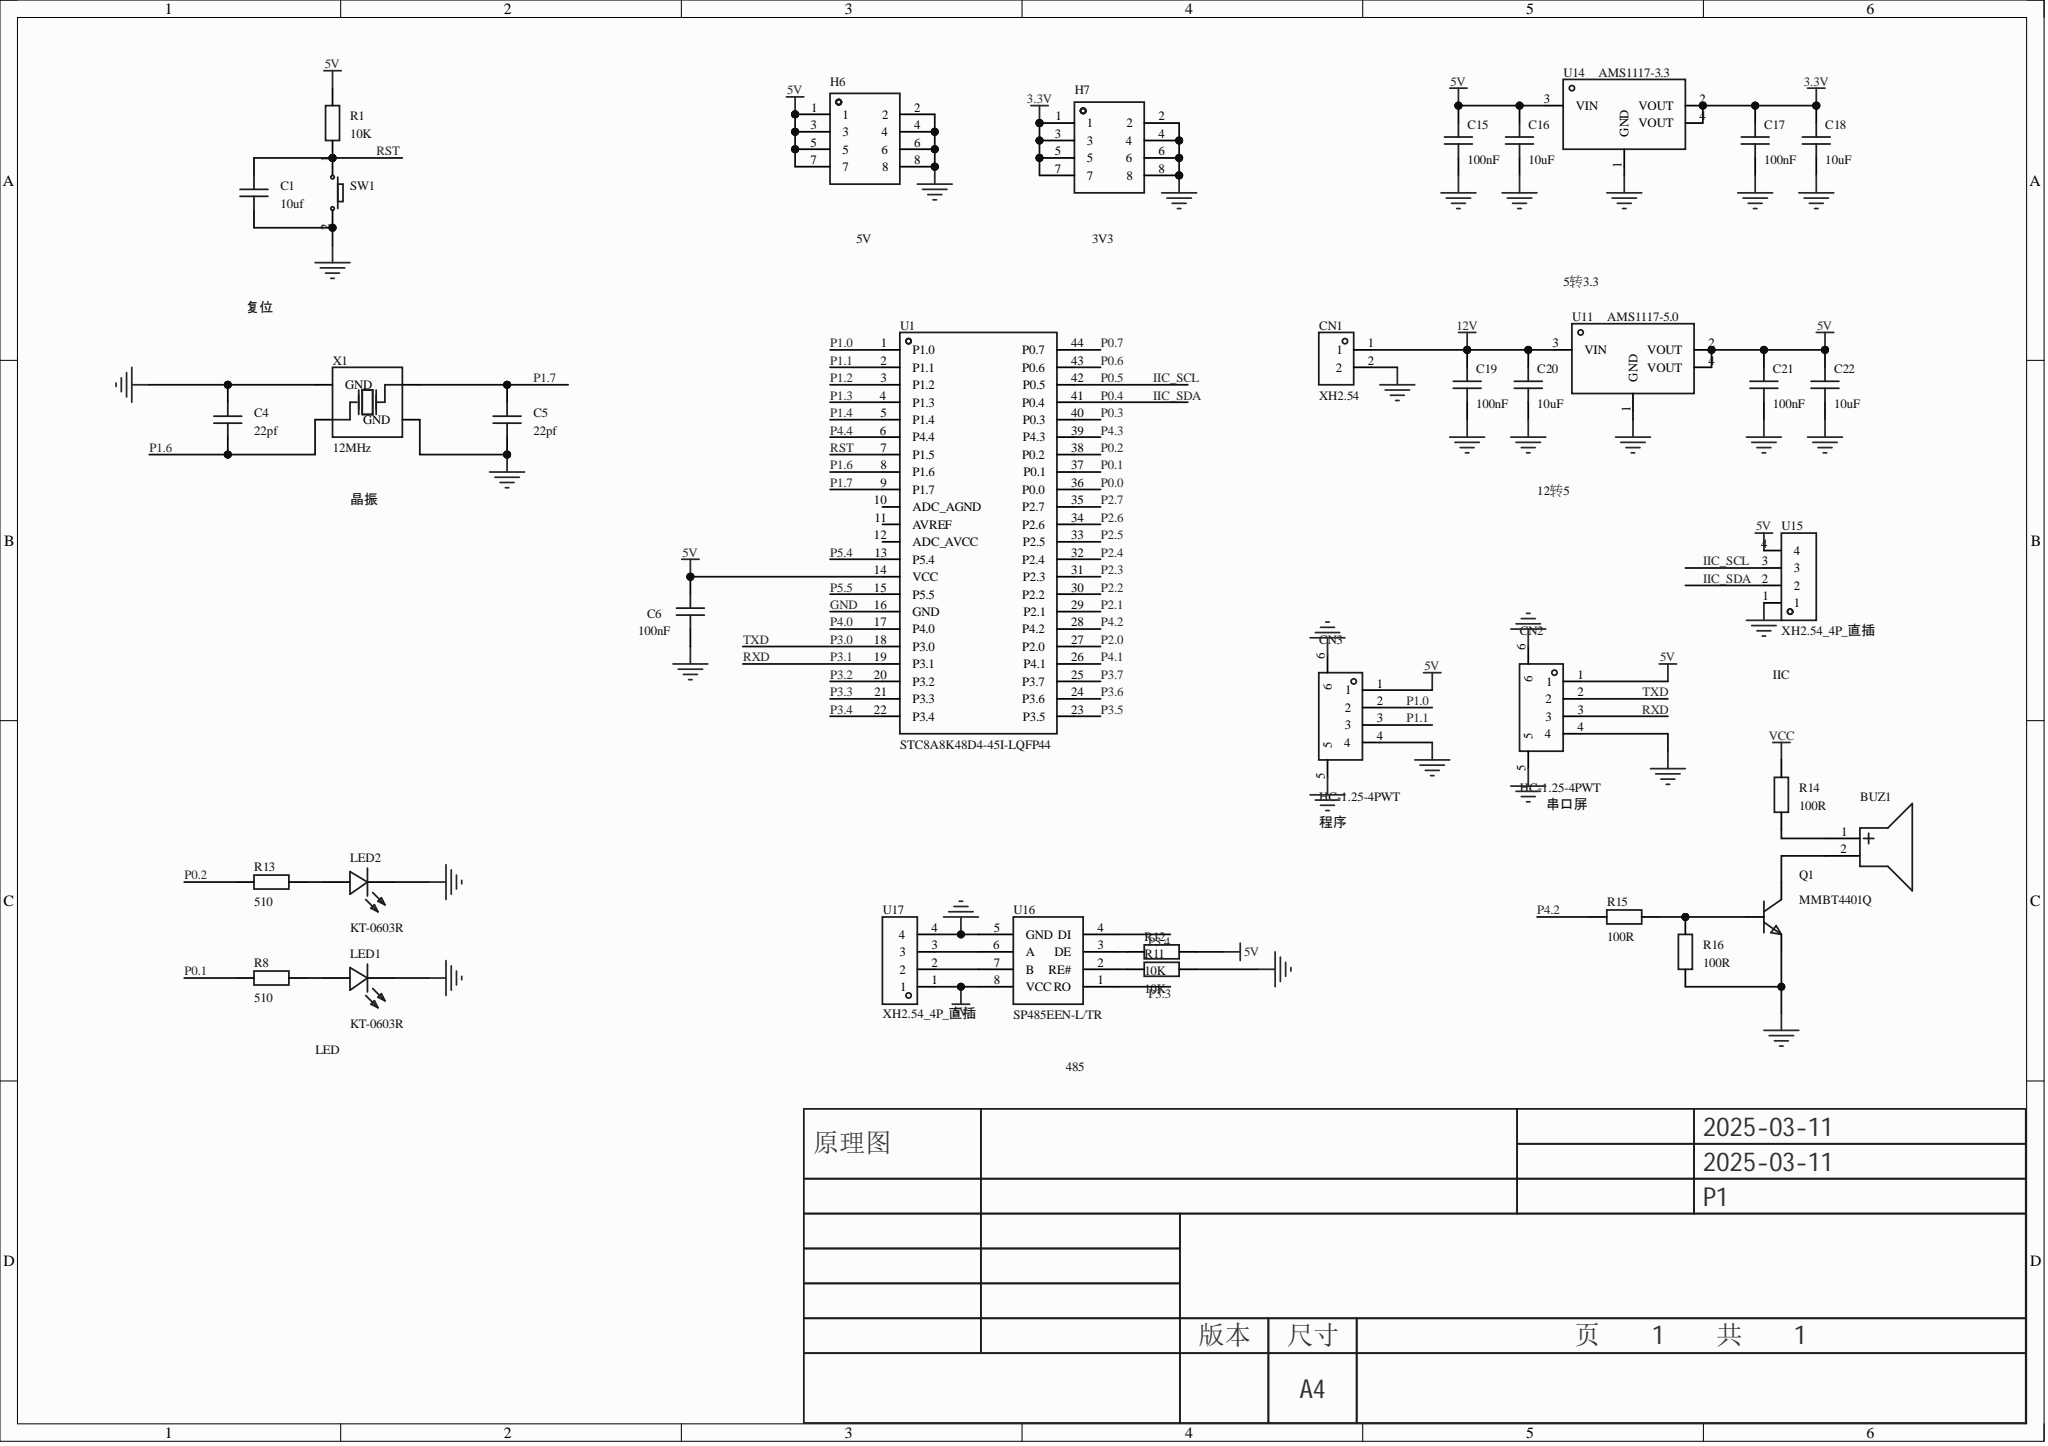Circuit board | Altium Designer | 37 parts | 27 nets
Bill of materials:
Comment,Description,Designator,Footprint,LibRef,Quantity
"","","BUZ1","BUZ-TH_BD12.0-P7.60-D0.6-FD","","1"
"10uf","","C1","C0805","CAP_0805","1"
"22pf","","C4, C5","C0805","CAP_0805","2"
"100nF","","C6","C0805","CAP_0805","1"
"100nF","","C15, C17, C19, C21","C0603","CAP_0603","4"
"10uF","","C16, C18, C20, C22","C0603","CAP_0603","4"
"XH2.54","","CN1","CONN-TH_XH2.54-2P","XH2.54-2PIN-直针","1"
"HC-1.25-4PWT","插针结构:1x4P;间距:1.25mm;安装方式:卧贴;参考系列:PicoBlade(MX 1.25);总PIN数:4P;排数:1;每排PIN数:4;行距:-;额定电流:1A;触头材质:黄铜;触头镀层:锡;工作温度范围:-40℃~+105℃;","CN2, CN3","CONN-SMD_4P-P1.25-HC-1.25-4PWT","HC-1.25-4PWT","2"
"","","H6, H7","HDR-TH_8P-P2.54-V-M-R2-C4-S2.54","HDR-M_2.54_2x4","2"
"KT-0603R","发光颜色:红色;功率:-;正向电流:-;主波长:-;二极管配置:-;透镜颜色:-;色温:-;发光角度:-;载带方式:-;工作温度:-40℃~+85℃;","LED1, LED2","LED0603-RD","KT-0603R","2"
"MMBT4401Q","晶体管类型:NPN;集电极电流(Ic):600mA;集射极击穿电压(Vceo):40V;耗散功率(Pd):300mW;直流电流增益(hFE):100@150mA,1V;","Q1","SOT-23-3_L2.9-W1.3-P1.90-LS2.4-BR","MMBT4401Q","1"
"10K","","R1, R11, R12","R0805","Res_0805","3"
"510","","R8, R13","R0603","Res_0603","2"
"100R","","R14, R15, R16","R0805","Res_0805","3"
"","","SW1","Key_SMD_3x4x2","Key_SMD_3x4x2","1"
"STC8A8K48D4-45I-LQFP44","","U1","LQFP-44_L10.0-W10.0-P0.80-LS12.0-BL","STC8A8K48D4-45I-LQFP44","1"
"AMS1117-5.0","输出类型:固定;工作电压:12V;输出电压:5V;输出电流:1A;电源纹波抑制比(PSRR):-;输出极性:正极;","U11","SOT-223_L6.5-W3.5-P2.30-LS7.0-BR","AMS1117-5.0_C6187","1"
"AMS1117-3.3","输出类型:固定;工作电压:-;输出电压:3.3V;输出电流:1A;电源纹波抑制比(PSRR):72dB@(120Hz);输出极性:正极;","U14","SOT-223-3_L6.5-W3.4-P2.30-LS7.0-BR","AMS1117-3.3_C6186","1"
"XH2.54_4P_直插","","U15, U17","CONN-TH_4P-P2.50-XH2.54-4P","XH2.54_4P_直插","2"
"SP485EEN-L/TR","类型:收发器;数据速率:10Mbps;","U16","SOIC-8_L5.0-W4.0-P1.27-LS6.0-BL","SP485EEN-L/TR","1"
"12MHz","晶振类型:贴片晶振;频率:12MHz;常温频差:±20ppm;外接负载电容:18pF;频率稳定度(全温):±20ppm;","X1","OSC-SMD_4P-L3.2-W2.5-BL","7M12000039","1"
Netlist (Protel format):
[
BUZ1
BUZ-TH_BD12.0-P7.60-D0.6-FD
5VDC???,F12,??7.6



]
[
C1
C0805
10uf



]
[
C4
C0805
22pf



]
[
C5
C0805
22pf



]
[
C6
C0805
100nF



]
[
C15
C0603
100nF



]
[
C16
C0603
10uF



]
[
C17
C0603
100nF



]
[
C18
C0603
10uF



]
[
C19
C0603
100nF



]
[
C20
C0603
10uF



]
[
C21
C0603
100nF



]
[
C22
C0603
10uF



]
[
CN1
CONN-TH_XH2.54-2P
XH2.54



]
[
CN2
CONN-SMD_4P-P1.25-HC-1.25-4PWT
HC-1.25-4PWT



]
[
CN3
CONN-SMD_4P-P1.25-HC-1.25-4PWT
HC-1.25-4PWT



]
[
H6
HDR-TH_8P-P2.54-V-M-R2-C4-S2.54




]
[
H7
HDR-TH_8P-P2.54-V-M-R2-C4-S2.54




]
[
LED1
LED0603-RD
KT-0603R



]
[
LED2
LED0603-RD
KT-0603R



]
[
Q1
SOT-23-3_L2.9-W1.3-P1.90-LS2.4-BR
MMBT4401Q



]
[
R1
R0805
10K



]
[
R8
R0603
510



]
[
R11
R0805
10K



]
[
R12
R0805
10K



]
[
R13
R0603
510



]
[
R14
R0805
100R



]
[
R15
R0805
100R



]
[
R16
R0805
100R



]
[
SW1
Key_SMD_3x4x2




]
[
U1
LQFP-44_L10.0-W10.0-P0.80-LS12.0-BL
STC8A8K48D4-45I-LQFP44



]
[
U11
SOT-223_L6.5-W3.5-P2.30-LS7.0-BR
AMS1117-5.0



]
[
U14
SOT-223-3_L6.5-W3.4-P2.30-LS7.0-BR
AMS1117-3.3



]
[
U15
CONN-TH_4P-P2.50-XH2.54-4P
XH2.54_4P_直插



]
[
U16
SOIC-8_L5.0-W4.0-P1.27-LS6.0-BL
SP485EEN-L/TR



]
[
U17
CONN-TH_4P-P2.50-XH2.54-4P
XH2.54_4P_直插



]
[
X1
OSC-SMD_4P-L3.2-W2.5-BL
12MHz



]
(
RST
C1-1
R1-2
SW1-1
U1-7
)
(
P4.2
R15-1
U1-28
)
(
P3.4
U1-22
U16-4
)
(
P3.3
U1-21
U16-1
)
(
P3.1
CN2-3
U1-19
)
(
P3.0
CN2-2
U1-18
)
(
P1.7
C5-2
U1-9
X1-3
)
(
P1.6
C4-1
U1-8
X1-1
)
(
P1.1
CN3-3
U1-2
)
(
P1.0
CN3-2
U1-1
)
(
P0.2
R13-1
U1-38
)
(
P0.1
R8-1
U1-37
)
(
NetU16_7
U16-7
U17-2
)
(
NetU16_6
U16-6
U17-3
)
(
NetR12_1
R12-1
U16-3
)
(
NetR11_1
R11-1
U16-2
)
(
NetQ1_1
Q1-1
R15-2
R16-1
)
(
NetLED2_2
LED2-2
R13-2
)
(
NetLED1_2
LED1-2
R8-2
)
(
NetBUZ1_2
BUZ1-2
Q1-3
)
(
NetBUZ1_1
BUZ1-1
R14-2
)
(
IIC_SDA
U1-41
U15-2
)
(
IIC_SCL
U1-42
U15-3
)
(
GND
C1-2
C4-2
C5-1
C6-1
C15-1
C16-1
C17-1
C18-1
C19-1
C20-1
C21-1
C22-1
CN1-2
CN2-4
CN2-5
CN2-6
CN3-4
CN3-5
CN3-6
H6-2
H6-4
H6-6
H6-8
H7-2
H7-4
H7-6
H7-8
LED1-1
LED2-1
Q1-2
R11-2
R16-2
SW1-2
U1-16
U11-1
U14-1
U15-1
U16-5
U17-4
X1-2
X1-4
)
(
12V
C19-2
C20-2
CN1-1
U11-3
)
(
5V
C6-2
C15-2
C16-2
C21-2
C22-2
CN2-1
CN3-1
H6-1
H6-3
H6-5
H6-7
R1-1
R12-2
U1-14
U11-2
U11-4
U14-3
U15-4
U16-8
U17-1
)
(
3.3V
C17-2
C18-2
H7-1
H7-3
H7-5
H7-7
U14-2
U14-4
)